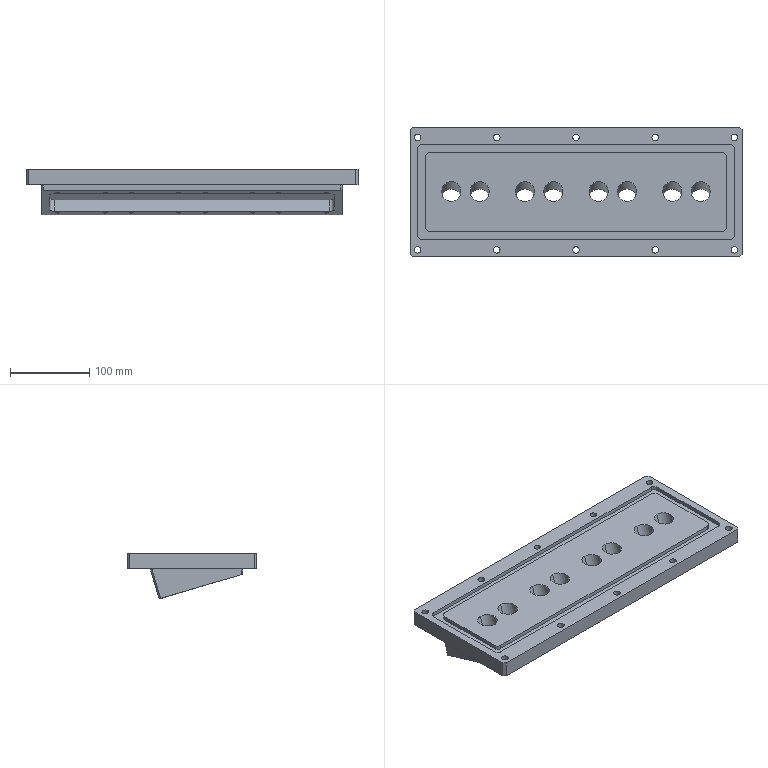Part | SolidWorks | features HoleWzd 3, ICE 3, Chamfer 2, Fillet 2, Extrusion 1 | 1 solid | 176 faces | box 419 x 164 x 57.82 mm | volume 1739257 mm3 | cylinder 100 | plane 44 | cone 32 | commonest cylinder face diameters 5 x32 8.4 x20 15 x20 24 x16 12 x12